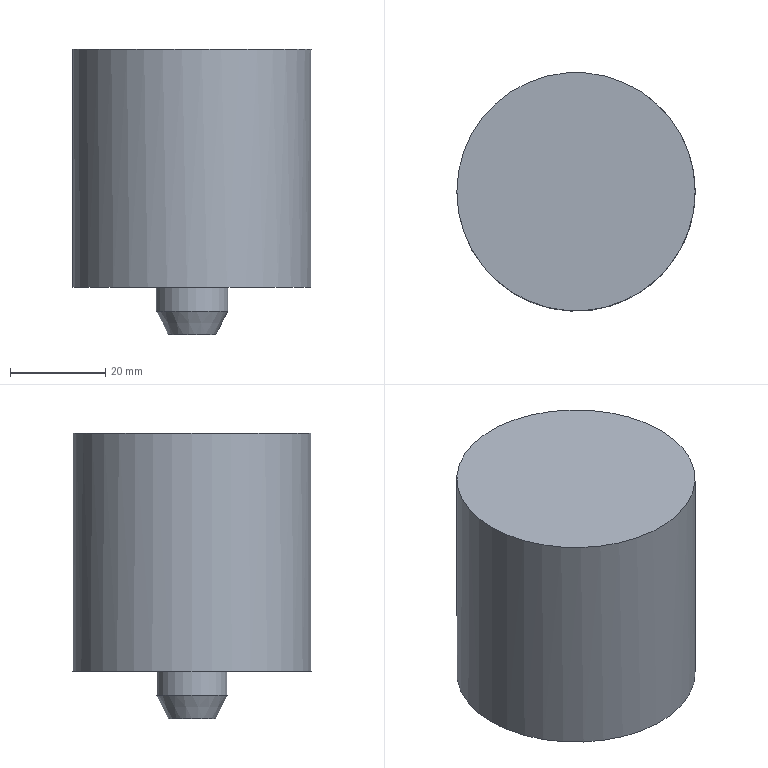Part | NX | features solid 2 | 1 solid | 6 faces | box 50 x 50 x 60 mm | volume 99680 mm3 | plane 3 | cylinder 2 | cone 1 | commonest cylinder face diameters 15 x1 50 x1
STEP:
#1=CARTESIAN_POINT('',(667.5,560.,-85.));
#2=VERTEX_POINT('',#1);
#3=CARTESIAN_POINT('',(675.,560.,-85.));
#4=DIRECTION('',(0.,0.,1.));
#5=DIRECTION('',(-1.,0.,0.));
#6=AXIS2_PLACEMENT_3D('',#3,#4,#5);
#7=CIRCLE('',#6,7.5);
#8=EDGE_CURVE('',#2,#2,#7,.T.);
#9=ORIENTED_EDGE('',*,*,#8,.T.);
#10=EDGE_LOOP('',(#9));
#11=FACE_BOUND('',#10,.T.);
#12=CARTESIAN_POINT('',(650.,560.,-85.));
#13=VERTEX_POINT('',#12);
#14=CARTESIAN_POINT('',(675.,560.,-85.));
#15=DIRECTION('',(0.,0.,-1.));
#16=DIRECTION('',(-1.,0.,0.));
#17=AXIS2_PLACEMENT_3D('',#14,#15,#16);
#18=CIRCLE('',#17,25.);
#19=EDGE_CURVE('',#13,#13,#18,.T.);
#20=ORIENTED_EDGE('',*,*,#19,.T.);
#21=EDGE_LOOP('',(#20));
#22=FACE_BOUND('',#21,.T.);
#23=CARTESIAN_POINT('',(675.,560.,-85.));
#24=DIRECTION('',(0.,0.,-1.));
#25=DIRECTION('',(-1.,0.,0.));
#26=AXIS2_PLACEMENT_3D('',#23,#24,#25);
#27=PLANE('',#26);
#28=ADVANCED_FACE('',(#11,#22),#27,.T.);
#29=CARTESIAN_POINT('',(700.,560.,-35.));
#30=VERTEX_POINT('',#29);
#31=CARTESIAN_POINT('',(675.,560.,-35.));
#32=DIRECTION('',(0.,0.,1.));
#33=DIRECTION('',(1.,0.,0.));
#34=AXIS2_PLACEMENT_3D('',#31,#32,#33);
#35=CIRCLE('',#34,25.);
#36=EDGE_CURVE('',#30,#30,#35,.T.);
#37=ORIENTED_EDGE('',*,*,#36,.T.);
#38=EDGE_LOOP('',(#37));
#39=FACE_BOUND('',#38,.T.);
#40=CARTESIAN_POINT('',(675.,560.,-35.));
#41=DIRECTION('',(0.,0.,1.));
#42=DIRECTION('',(1.,0.,0.));
#43=AXIS2_PLACEMENT_3D('',#40,#41,#42);
#44=PLANE('',#43);
#45=ADVANCED_FACE('',(#39),#44,.T.);
#46=ORIENTED_EDGE('',*,*,#19,.F.);
#47=EDGE_LOOP('',(#46));
#48=FACE_BOUND('',#47,.T.);
#49=ORIENTED_EDGE('',*,*,#36,.F.);
#50=EDGE_LOOP('',(#49));
#51=FACE_BOUND('',#50,.T.);
#52=CARTESIAN_POINT('',(675.,560.,-45.));
#53=DIRECTION('',(0.,0.,-1.));
#54=DIRECTION('',(-1.,0.,0.));
#55=AXIS2_PLACEMENT_3D('',#52,#53,#54);
#56=CYLINDRICAL_SURFACE('',#55,25.);
#57=ADVANCED_FACE('',(#48,#51),#56,.T.);
#58=CARTESIAN_POINT('',(682.5,560.,-90.));
#59=VERTEX_POINT('',#58);
#60=CARTESIAN_POINT('',(675.,560.,-90.));
#61=DIRECTION('',(0.,0.,-1.));
#62=DIRECTION('',(1.,0.,0.));
#63=AXIS2_PLACEMENT_3D('',#60,#61,#62);
#64=CIRCLE('',#63,7.5);
#65=EDGE_CURVE('',#59,#59,#64,.T.);
#66=ORIENTED_EDGE('',*,*,#65,.F.);
#67=EDGE_LOOP('',(#66));
#68=FACE_BOUND('',#67,.T.);
#69=ORIENTED_EDGE('',*,*,#8,.F.);
#70=EDGE_LOOP('',(#69));
#71=FACE_BOUND('',#70,.T.);
#72=CARTESIAN_POINT('',(675.,560.,-85.));
#73=DIRECTION('',(0.,0.,-1.));
#74=DIRECTION('',(-1.,0.,0.));
#75=AXIS2_PLACEMENT_3D('',#72,#73,#74);
#76=CYLINDRICAL_SURFACE('',#75,7.5);
#77=ADVANCED_FACE('',(#68,#71),#76,.T.);
#78=CARTESIAN_POINT('',(680.,560.,-95.));
#79=VERTEX_POINT('',#78);
#80=CARTESIAN_POINT('',(675.,560.,-95.));
#81=DIRECTION('',(0.,0.,-1.));
#82=DIRECTION('',(1.,0.,0.));
#83=AXIS2_PLACEMENT_3D('',#80,#81,#82);
#84=CIRCLE('',#83,5.);
#85=EDGE_CURVE('',#79,#79,#84,.T.);
#86=ORIENTED_EDGE('',*,*,#85,.T.);
#87=EDGE_LOOP('',(#86));
#88=FACE_BOUND('',#87,.T.);
#89=CARTESIAN_POINT('',(675.,560.,-95.));
#90=DIRECTION('',(0.,0.,-1.));
#91=DIRECTION('',(1.,0.,0.));
#92=AXIS2_PLACEMENT_3D('',#89,#90,#91);
#93=PLANE('',#92);
#94=ADVANCED_FACE('',(#88),#93,.T.);
#95=ORIENTED_EDGE('',*,*,#85,.F.);
#96=EDGE_LOOP('',(#95));
#97=FACE_BOUND('',#96,.T.);
#98=ORIENTED_EDGE('',*,*,#65,.T.);
#99=EDGE_LOOP('',(#98));
#100=FACE_BOUND('',#99,.T.);
#101=CARTESIAN_POINT('',(675.,560.,-90.));
#102=DIRECTION('',(0.,0.,1.));
#103=DIRECTION('',(-1.,0.,0.));
#104=AXIS2_PLACEMENT_3D('',#101,#102,#103);
#105=CONICAL_SURFACE('',#104,7.5,0.4636);
#106=ADVANCED_FACE('',(#97,#100),#105,.T.);
#107=CLOSED_SHELL('',(#28,#45,#57,#77,#94,#106));
#108=MANIFOLD_SOLID_BREP('',#107);
#109=(LENGTH_UNIT()NAMED_UNIT(*)SI_UNIT(.MILLI.,.METRE.));
#110=UNCERTAINTY_MEASURE_WITH_UNIT(LENGTH_MEASURE(0.00001),#109,'','');
#111=(NAMED_UNIT(*)PLANE_ANGLE_UNIT()SI_UNIT($,.RADIAN.));
#112=(NAMED_UNIT(*)SI_UNIT($,.STERADIAN.)SOLID_ANGLE_UNIT());
#113=(GEOMETRIC_REPRESENTATION_CONTEXT(3)GLOBAL_UNCERTAINTY_ASSIGNED_CONTEXT((#110))GLOBAL_UNIT_ASSIGNED_CONTEXT((#109,#111,#112))REPRESENTATION_CONTEXT('',''));
#114=ADVANCED_BREP_SHAPE_REPRESENTATION('',(#108),#113);